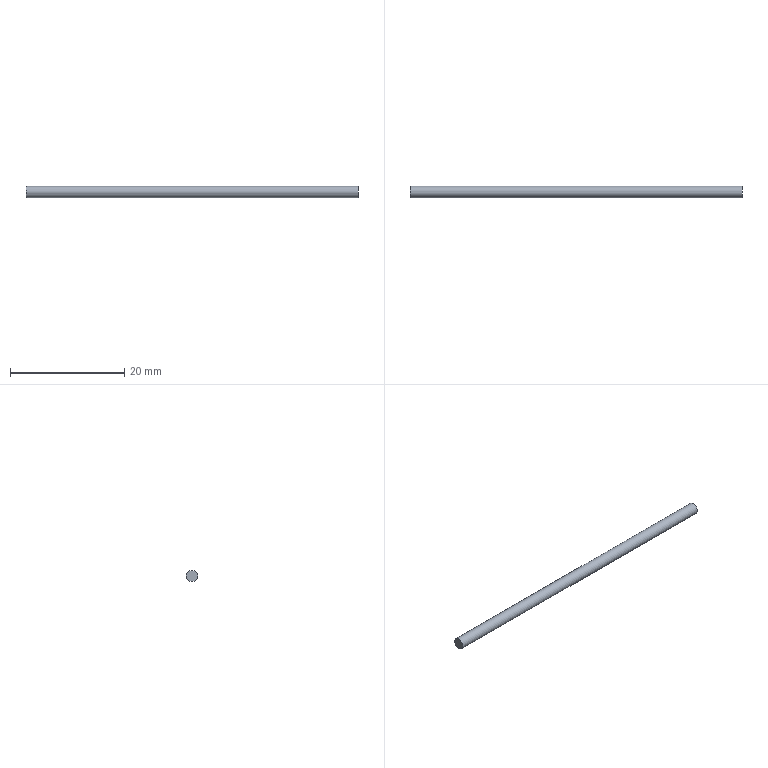Part | STEP file | 1-34 | 1 solid | 3 faces | box 58 x 2 x 2 mm | volume 182.212 mm3 | plane 2 | cylinder 1 | commonest cylinder face diameters 2 x1
STEP:
#1=CARTESIAN_POINT('',(0.,0.,0.));
#2=DIRECTION('',(0.,0.,1.));
#3=DIRECTION('',(1.,0.,0.));
#4=AXIS2_PLACEMENT_3D('',#1,#2,#3);
#5=CARTESIAN_POINT('',(-29.,1.,0.));
#6=VERTEX_POINT('',#5);
#7=CARTESIAN_POINT('',(-29.,0.,0.));
#8=DIRECTION('',(1.,0.,0.));
#9=DIRECTION('',(0.,1.,0.));
#10=AXIS2_PLACEMENT_3D('',#7,#8,#9);
#11=CIRCLE('',#10,1.);
#12=CARTESIAN_POINT('',(-29.,-0.2679,0.));
#13=DIRECTION('',(1.,0.,0.));
#14=DIRECTION('',(0.,1.,0.));
#15=AXIS2_PLACEMENT_3D('',#12,#13,#14);
#16=PLANE('',#15);
#17=CARTESIAN_POINT('',(0.2679,0.));
#18=DIRECTION('',(1.,0.));
#19=AXIS2_PLACEMENT_2D('',#17,#18);
#20=CIRCLE('',#19,1.);
#21=(GEOMETRIC_REPRESENTATION_CONTEXT(2)PARAMETRIC_REPRESENTATION_CONTEXT()REPRESENTATION_CONTEXT('',''));
#22=DEFINITIONAL_REPRESENTATION('',(#20),#21);
#23=PCURVE('',#16,#22);
#24=CARTESIAN_POINT('',(-29.,0.,0.));
#25=DIRECTION('',(1.,0.,0.));
#26=DIRECTION('',(0.,1.,0.));
#27=AXIS2_PLACEMENT_3D('',#24,#25,#26);
#28=CYLINDRICAL_SURFACE('',#27,1.);
#29=CARTESIAN_POINT('',(0.,0.));
#30=DIRECTION('',(1.,0.));
#31=VECTOR('',#30,1.);
#32=LINE('',#29,#31);
#33=(GEOMETRIC_REPRESENTATION_CONTEXT(2)PARAMETRIC_REPRESENTATION_CONTEXT()REPRESENTATION_CONTEXT('',''));
#34=DEFINITIONAL_REPRESENTATION('',(#32),#33);
#35=PCURVE('',#28,#34);
#36=SURFACE_CURVE('',#11,(#23,#35),.PCURVE_S1.);
#37=EDGE_CURVE('',#6,#6,#36,.T.);
#38=ORIENTED_EDGE('',*,*,#37,.T.);
#39=EDGE_LOOP('',(#38));
#40=FACE_BOUND('',#39,.F.);
#41=ADVANCED_FACE('',(#40),#16,.F.);
#42=CARTESIAN_POINT('',(29.,1.,0.));
#43=VERTEX_POINT('',#42);
#44=CARTESIAN_POINT('',(29.,0.,0.));
#45=DIRECTION('',(1.,0.,0.));
#46=DIRECTION('',(0.,1.,0.));
#47=AXIS2_PLACEMENT_3D('',#44,#45,#46);
#48=CIRCLE('',#47,1.);
#49=CARTESIAN_POINT('',(29.,-0.2679,0.));
#50=DIRECTION('',(1.,0.,0.));
#51=DIRECTION('',(0.,1.,0.));
#52=AXIS2_PLACEMENT_3D('',#49,#50,#51);
#53=PLANE('',#52);
#54=CARTESIAN_POINT('',(0.2679,0.));
#55=DIRECTION('',(1.,0.));
#56=AXIS2_PLACEMENT_2D('',#54,#55);
#57=CIRCLE('',#56,1.);
#58=(GEOMETRIC_REPRESENTATION_CONTEXT(2)PARAMETRIC_REPRESENTATION_CONTEXT()REPRESENTATION_CONTEXT('',''));
#59=DEFINITIONAL_REPRESENTATION('',(#57),#58);
#60=PCURVE('',#53,#59);
#61=CARTESIAN_POINT('',(0.,58.));
#62=DIRECTION('',(1.,0.));
#63=VECTOR('',#62,1.);
#64=LINE('',#61,#63);
#65=(GEOMETRIC_REPRESENTATION_CONTEXT(2)PARAMETRIC_REPRESENTATION_CONTEXT()REPRESENTATION_CONTEXT('',''));
#66=DEFINITIONAL_REPRESENTATION('',(#64),#65);
#67=PCURVE('',#28,#66);
#68=SURFACE_CURVE('',#48,(#60,#67),.PCURVE_S1.);
#69=EDGE_CURVE('',#43,#43,#68,.T.);
#70=ORIENTED_EDGE('',*,*,#69,.T.);
#71=EDGE_LOOP('',(#70));
#72=FACE_BOUND('',#71,.T.);
#73=ADVANCED_FACE('',(#72),#53,.T.);
#74=ORIENTED_EDGE('',*,*,#37,.T.);
#75=CARTESIAN_POINT('',(-29.,1.,0.));
#76=DIRECTION('',(1.,0.,0.));
#77=VECTOR('',#76,1.);
#78=LINE('',#75,#77);
#79=CARTESIAN_POINT('',(6.283,0.));
#80=DIRECTION('',(0.,1.));
#81=VECTOR('',#80,1.);
#82=LINE('',#79,#81);
#83=(GEOMETRIC_REPRESENTATION_CONTEXT(2)PARAMETRIC_REPRESENTATION_CONTEXT()REPRESENTATION_CONTEXT('',''));
#84=DEFINITIONAL_REPRESENTATION('',(#82),#83);
#85=PCURVE('',#28,#84);
#86=CARTESIAN_POINT('',(0.,0.));
#87=DIRECTION('',(0.,1.));
#88=VECTOR('',#87,1.);
#89=LINE('',#86,#88);
#90=(GEOMETRIC_REPRESENTATION_CONTEXT(2)PARAMETRIC_REPRESENTATION_CONTEXT()REPRESENTATION_CONTEXT('',''));
#91=DEFINITIONAL_REPRESENTATION('',(#89),#90);
#92=PCURVE('',#28,#91);
#93=SEAM_CURVE('',#78,(#85,#92),.PCURVE_S1.);
#94=EDGE_CURVE('',#6,#43,#93,.T.);
#95=ORIENTED_EDGE('',*,*,#94,.T.);
#96=ORIENTED_EDGE('',*,*,#69,.F.);
#97=ORIENTED_EDGE('',*,*,#94,.F.);
#98=EDGE_LOOP('',(#74,#95,#96,#97));
#99=FACE_BOUND('',#98,.T.);
#100=ADVANCED_FACE('',(#99),#28,.T.);
#101=CLOSED_SHELL('',(#41,#73,#100));
#102=MANIFOLD_SOLID_BREP('',#101);
#103=(LENGTH_UNIT()NAMED_UNIT(*)SI_UNIT(.MILLI.,.METRE.));
#104=UNCERTAINTY_MEASURE_WITH_UNIT(LENGTH_MEASURE(0.0000001),#103,'','');
#105=(NAMED_UNIT(*)PLANE_ANGLE_UNIT()SI_UNIT($,.RADIAN.));
#106=(NAMED_UNIT(*)SI_UNIT($,.STERADIAN.)SOLID_ANGLE_UNIT());
#107=(GEOMETRIC_REPRESENTATION_CONTEXT(3)GLOBAL_UNCERTAINTY_ASSIGNED_CONTEXT((#104))GLOBAL_UNIT_ASSIGNED_CONTEXT((#103,#105,#106))REPRESENTATION_CONTEXT('',''));
#108=ADVANCED_BREP_SHAPE_REPRESENTATION('',(#4,#102),#107);